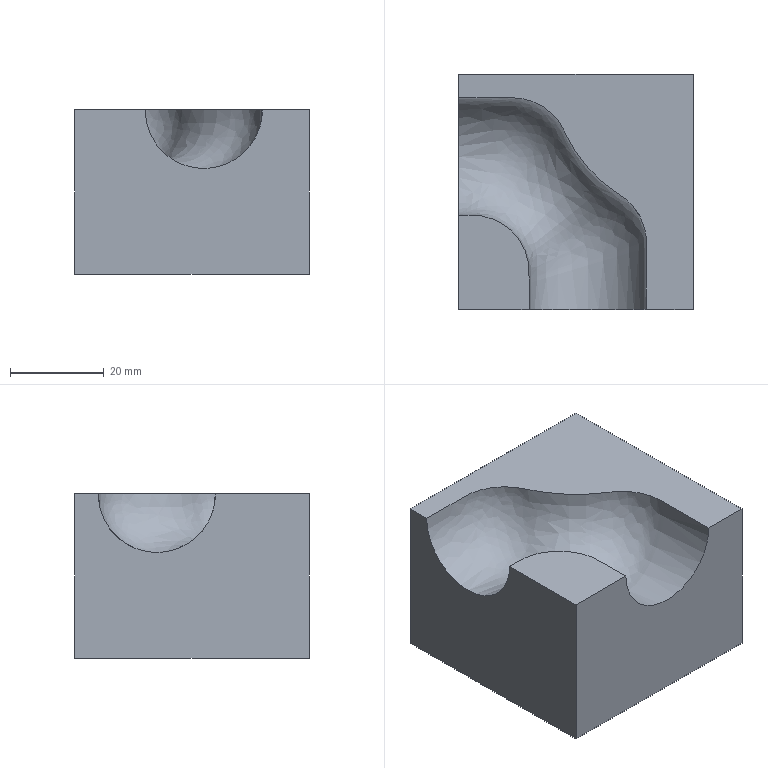Part | NX | 1 solid | 8 faces | box 50 x 50 x 35 mm | volume 75885 mm3 | plane 7 | spline 1
STEP:
#1=CARTESIAN_POINT('',(0.,45.,0.));
#2=VERTEX_POINT('',#1);
#3=CARTESIAN_POINT('',(0.,20.,0.));
#4=VERTEX_POINT('',#3);
#5=CARTESIAN_POINT('',(0.,45.,0.));
#6=CARTESIAN_POINT('',(0.,45.,-3.284));
#7=CARTESIAN_POINT('',(0.,42.295,-9.786));
#8=CARTESIAN_POINT('',(0.,32.5,-13.857));
#9=CARTESIAN_POINT('',(0.,22.705,-9.785));
#10=CARTESIAN_POINT('',(0.,20.,-3.285));
#11=CARTESIAN_POINT('',(0.,20.,0.));
#12=B_SPLINE_CURVE_WITH_KNOTS('',3,(#5,#6,#7,#8,#9,#10,#11),.UNSPECIFIED.,.F.,.F.,(4,1,1,1,4),(0.,0.25,0.5,0.75,1.),.UNSPECIFIED.);
#13=EDGE_CURVE('',#2,#4,#12,.T.);
#14=ORIENTED_EDGE('',*,*,#13,.F.);
#15=CARTESIAN_POINT('',(0.,50.,0.));
#16=VERTEX_POINT('',#15);
#17=CARTESIAN_POINT('',(0.,0.,0.));
#18=DIRECTION('',(0.,1.,0.));
#19=VECTOR('',#18,1000.);
#20=LINE('',#17,#19);
#21=EDGE_CURVE('',#2,#16,#20,.T.);
#22=ORIENTED_EDGE('',*,*,#21,.T.);
#23=CARTESIAN_POINT('',(0.,50.,-35.));
#24=VERTEX_POINT('',#23);
#25=CARTESIAN_POINT('',(0.,50.,-35.));
#26=DIRECTION('',(0.,0.,1.));
#27=VECTOR('',#26,1000.);
#28=LINE('',#25,#27);
#29=EDGE_CURVE('',#24,#16,#28,.T.);
#30=ORIENTED_EDGE('',*,*,#29,.F.);
#31=CARTESIAN_POINT('',(0.,0.,-35.));
#32=VERTEX_POINT('',#31);
#33=CARTESIAN_POINT('',(0.,0.,-35.));
#34=DIRECTION('',(0.,1.,0.));
#35=VECTOR('',#34,1000.);
#36=LINE('',#33,#35);
#37=EDGE_CURVE('',#32,#24,#36,.T.);
#38=ORIENTED_EDGE('',*,*,#37,.F.);
#39=CARTESIAN_POINT('',(0.,0.,0.));
#40=VERTEX_POINT('',#39);
#41=CARTESIAN_POINT('',(0.,0.,-35.));
#42=DIRECTION('',(0.,0.,1.));
#43=VECTOR('',#42,1000.);
#44=LINE('',#41,#43);
#45=EDGE_CURVE('',#32,#40,#44,.T.);
#46=ORIENTED_EDGE('',*,*,#45,.T.);
#47=CARTESIAN_POINT('',(0.,0.,0.));
#48=DIRECTION('',(0.,1.,0.));
#49=VECTOR('',#48,1000.);
#50=LINE('',#47,#49);
#51=EDGE_CURVE('',#40,#4,#50,.T.);
#52=ORIENTED_EDGE('',*,*,#51,.T.);
#53=EDGE_LOOP('',(#14,#22,#30,#38,#46,#52));
#54=FACE_BOUND('',#53,.T.);
#55=CARTESIAN_POINT('',(0.,0.,-35.));
#56=DIRECTION('',(1.,0.,0.));
#57=DIRECTION('',(0.,0.,-1.));
#58=AXIS2_PLACEMENT_3D('',#55,#56,#57);
#59=PLANE('',#58);
#60=ADVANCED_FACE('',(#54),#59,.F.);
#61=CARTESIAN_POINT('',(15.,0.,0.));
#62=VERTEX_POINT('',#61);
#63=CARTESIAN_POINT('',(40.,0.,0.));
#64=VERTEX_POINT('',#63);
#65=CARTESIAN_POINT('',(15.,0.,0.));
#66=CARTESIAN_POINT('',(15.,0.,-3.284));
#67=CARTESIAN_POINT('',(17.705,0.,-9.786));
#68=CARTESIAN_POINT('',(27.5,0.,-13.857));
#69=CARTESIAN_POINT('',(37.295,0.,-9.785));
#70=CARTESIAN_POINT('',(40.,0.,-3.285));
#71=CARTESIAN_POINT('',(40.,0.,0.));
#72=B_SPLINE_CURVE_WITH_KNOTS('',3,(#65,#66,#67,#68,#69,#70,#71),.UNSPECIFIED.,.F.,.F.,(4,1,1,1,4),(0.,0.25,0.5,0.75,1.),.UNSPECIFIED.);
#73=EDGE_CURVE('',#62,#64,#72,.T.);
#74=ORIENTED_EDGE('',*,*,#73,.F.);
#75=CARTESIAN_POINT('',(50.,0.,0.));
#76=DIRECTION('',(-1.,0.,0.));
#77=VECTOR('',#76,1000.);
#78=LINE('',#75,#77);
#79=EDGE_CURVE('',#62,#40,#78,.T.);
#80=ORIENTED_EDGE('',*,*,#79,.T.);
#81=ORIENTED_EDGE('',*,*,#45,.F.);
#82=CARTESIAN_POINT('',(50.,0.,-35.));
#83=VERTEX_POINT('',#82);
#84=CARTESIAN_POINT('',(50.,0.,-35.));
#85=DIRECTION('',(-1.,0.,0.));
#86=VECTOR('',#85,1000.);
#87=LINE('',#84,#86);
#88=EDGE_CURVE('',#83,#32,#87,.T.);
#89=ORIENTED_EDGE('',*,*,#88,.F.);
#90=CARTESIAN_POINT('',(50.,0.,0.));
#91=VERTEX_POINT('',#90);
#92=CARTESIAN_POINT('',(50.,0.,-35.));
#93=DIRECTION('',(0.,0.,1.));
#94=VECTOR('',#93,1000.);
#95=LINE('',#92,#94);
#96=EDGE_CURVE('',#83,#91,#95,.T.);
#97=ORIENTED_EDGE('',*,*,#96,.T.);
#98=CARTESIAN_POINT('',(50.,0.,0.));
#99=DIRECTION('',(-1.,0.,0.));
#100=VECTOR('',#99,1000.);
#101=LINE('',#98,#100);
#102=EDGE_CURVE('',#91,#64,#101,.T.);
#103=ORIENTED_EDGE('',*,*,#102,.T.);
#104=EDGE_LOOP('',(#74,#80,#81,#89,#97,#103));
#105=FACE_BOUND('',#104,.T.);
#106=CARTESIAN_POINT('',(50.,0.,-35.));
#107=DIRECTION('',(0.,1.,0.));
#108=DIRECTION('',(0.,0.,1.));
#109=AXIS2_PLACEMENT_3D('',#106,#107,#108);
#110=PLANE('',#109);
#111=ADVANCED_FACE('',(#105),#110,.F.);
#112=CARTESIAN_POINT('',(40.,0.,0.));
#113=CARTESIAN_POINT('',(40.,1.458,0.));
#114=CARTESIAN_POINT('',(39.999,4.376,0.));
#115=CARTESIAN_POINT('',(40.004,8.74,0.));
#116=CARTESIAN_POINT('',(39.987,12.414,0.));
#117=CARTESIAN_POINT('',(40.023,15.271,0.));
#118=CARTESIAN_POINT('',(39.51,18.133,0.));
#119=CARTESIAN_POINT('',(38.178,20.879,0.));
#120=CARTESIAN_POINT('',(36.19,23.093,0.));
#121=CARTESIAN_POINT('',(34.482,24.36,0.));
#122=CARTESIAN_POINT('',(32.637,25.485,0.));
#123=CARTESIAN_POINT('',(30.334,27.273,0.));
#124=CARTESIAN_POINT('',(27.665,29.806,0.));
#125=CARTESIAN_POINT('',(24.955,33.288,0.));
#126=CARTESIAN_POINT('',(23.146,36.496,0.));
#127=CARTESIAN_POINT('',(22.035,39.067,0.));
#128=CARTESIAN_POINT('',(20.341,41.437,0.));
#129=CARTESIAN_POINT('',(17.954,43.369,0.));
#130=CARTESIAN_POINT('',(15.201,44.519,0.));
#131=CARTESIAN_POINT('',(13.382,44.9,0.));
#132=CARTESIAN_POINT('',(12.299,44.987,0.));
#133=CARTESIAN_POINT('',(11.768,44.999,0.));
#134=CARTESIAN_POINT('',(11.654,45.,0.));
#135=CARTESIAN_POINT('',(11.403,45.,0.));
#136=CARTESIAN_POINT('',(11.323,45.,0.));
#137=CARTESIAN_POINT('',(10.876,45.,0.));
#138=CARTESIAN_POINT('',(10.783,45.,0.));
#139=CARTESIAN_POINT('',(10.487,45.,0.));
#140=CARTESIAN_POINT('',(10.089,45.,0.));
#141=CARTESIAN_POINT('',(9.59,45.,0.));
#142=CARTESIAN_POINT('',(9.175,45.,0.));
#143=CARTESIAN_POINT('',(8.953,45.,0.));
#144=CARTESIAN_POINT('',(8.694,45.,0.));
#145=CARTESIAN_POINT('',(8.757,45.,0.));
#146=CARTESIAN_POINT('',(8.722,45.,0.));
#147=CARTESIAN_POINT('',(8.699,45.,0.));
#148=CARTESIAN_POINT('',(8.596,45.,0.));
#149=CARTESIAN_POINT('',(8.419,45.,0.));
#150=CARTESIAN_POINT('',(8.089,45.,0.));
#151=CARTESIAN_POINT('',(7.511,45.,0.));
#152=CARTESIAN_POINT('',(6.231,45.,0.));
#153=CARTESIAN_POINT('',(3.964,45.,0.));
#154=CARTESIAN_POINT('',(1.44,45.,0.));
#155=CARTESIAN_POINT('',(0.,45.,0.));
#156=B_SPLINE_CURVE_WITH_KNOTS('',3,(#112,#113,#114,#115,#116,#117,#118,#119,#120,#121,#122,#123,#124,#125,#126,#127,#128,#129,#130,#131,#132,#133,#134,#135,#136,#137,#138,#139,#140,#141,#142,#143,#144,#145,#146,#147,#148,#149,#150,#151,#152,#153,#154,#155),.UNSPECIFIED.,.F.,.F.,(4,1,1,1,1,1,1,1,1,1,1,1,1,1,1,1,1,1,1,1,1,1,1,1,1,1,1,1,1,1,1,1,1,1,1,1,1,1,1,1,1,4),(0.,0.0625,0.125,0.1875,0.2188,0.25,0.3125,0.3438,0.375,0.4062,0.4375,0.5,0.5625,0.625,0.6562,0.6875,0.75,0.7812,0.8125,0.8281,0.832,0.834,0.8359,0.8398,0.8438,0.8477,0.8516,0.8594,0.8672,0.8711,0.873,0.875,0.877,0.8789,0.8828,0.8906,0.8984,0.9062,0.9219,0.9375,0.9688,1.),.UNSPECIFIED.);
#157=EDGE_CURVE('',#64,#2,#156,.T.);
#158=ORIENTED_EDGE('',*,*,#157,.F.);
#159=ORIENTED_EDGE('',*,*,#102,.F.);
#160=CARTESIAN_POINT('',(50.,50.,0.));
#161=VERTEX_POINT('',#160);
#162=CARTESIAN_POINT('',(50.,50.,0.));
#163=DIRECTION('',(0.,-1.,0.));
#164=VECTOR('',#163,1000.);
#165=LINE('',#162,#164);
#166=EDGE_CURVE('',#161,#91,#165,.T.);
#167=ORIENTED_EDGE('',*,*,#166,.F.);
#168=CARTESIAN_POINT('',(0.,50.,0.));
#169=DIRECTION('',(1.,0.,0.));
#170=VECTOR('',#169,1000.);
#171=LINE('',#168,#170);
#172=EDGE_CURVE('',#16,#161,#171,.T.);
#173=ORIENTED_EDGE('',*,*,#172,.F.);
#174=ORIENTED_EDGE('',*,*,#21,.F.);
#175=EDGE_LOOP('',(#158,#159,#167,#173,#174));
#176=FACE_BOUND('',#175,.T.);
#177=CARTESIAN_POINT('',(0.,0.,0.));
#178=DIRECTION('',(0.,0.,-1.));
#179=DIRECTION('',(-1.,0.,0.));
#180=AXIS2_PLACEMENT_3D('',#177,#178,#179);
#181=PLANE('',#180);
#182=ADVANCED_FACE('',(#176),#181,.F.);
#183=CARTESIAN_POINT('',(0.,20.,0.));
#184=CARTESIAN_POINT('',(0.6111,20.,0.));
#185=CARTESIAN_POINT('',(1.299,20.,0.));
#186=CARTESIAN_POINT('',(1.721,20.,0.));
#187=CARTESIAN_POINT('',(1.816,20.,0.));
#188=CARTESIAN_POINT('',(1.869,20.,0.));
#189=CARTESIAN_POINT('',(1.82,20.,0.));
#190=CARTESIAN_POINT('',(2.046,20.,0.));
#191=CARTESIAN_POINT('',(2.228,20.,0.));
#192=CARTESIAN_POINT('',(2.451,20.,0.));
#193=CARTESIAN_POINT('',(2.671,20.,0.));
#194=CARTESIAN_POINT('',(2.758,20.,0.));
#195=CARTESIAN_POINT('',(3.091,20.,0.));
#196=CARTESIAN_POINT('',(3.275,19.998,0.));
#197=CARTESIAN_POINT('',(4.143,19.968,0.));
#198=CARTESIAN_POINT('',(5.388,19.803,0.));
#199=CARTESIAN_POINT('',(7.194,19.298,0.));
#200=CARTESIAN_POINT('',(8.927,18.493,0.));
#201=CARTESIAN_POINT('',(11.094,17.03,0.));
#202=CARTESIAN_POINT('',(12.874,15.033,0.));
#203=CARTESIAN_POINT('',(14.073,12.756,0.));
#204=CARTESIAN_POINT('',(14.575,11.265,0.));
#205=CARTESIAN_POINT('',(14.825,10.105,0.));
#206=CARTESIAN_POINT('',(14.949,9.227,0.));
#207=CARTESIAN_POINT('',(14.992,8.526,0.));
#208=CARTESIAN_POINT('',(14.999,8.182,0.));
#209=CARTESIAN_POINT('',(15.,7.905,0.));
#210=CARTESIAN_POINT('',(15.,7.79,0.));
#211=CARTESIAN_POINT('',(15.,7.632,0.));
#212=CARTESIAN_POINT('',(15.,7.418,0.));
#213=CARTESIAN_POINT('',(15.,7.473,0.));
#214=CARTESIAN_POINT('',(15.,7.446,0.));
#215=CARTESIAN_POINT('',(15.,7.43,0.));
#216=CARTESIAN_POINT('',(15.,7.316,0.));
#217=CARTESIAN_POINT('',(15.,7.026,0.));
#218=CARTESIAN_POINT('',(15.,6.439,0.));
#219=CARTESIAN_POINT('',(15.,5.35,0.));
#220=CARTESIAN_POINT('',(15.,3.409,0.));
#221=CARTESIAN_POINT('',(15.,1.239,0.));
#222=CARTESIAN_POINT('',(15.,0.,0.));
#223=B_SPLINE_CURVE_WITH_KNOTS('',3,(#183,#184,#185,#186,#187,#188,#189,#190,#191,#192,#193,#194,#195,#196,#197,#198,#199,#200,#201,#202,#203,#204,#205,#206,#207,#208,#209,#210,#211,#212,#213,#214,#215,#216,#217,#218,#219,#220,#221,#222),.UNSPECIFIED.,.F.,.F.,(4,1,1,1,1,1,1,1,1,1,1,1,1,1,1,1,1,1,1,1,1,1,1,1,1,1,1,1,1,1,1,1,1,1,1,1,1,4),(0.,0.03125,0.04688,0.05469,0.05859,0.0625,0.06641,0.07031,0.07812,0.08594,0.09375,0.1016,0.1094,0.125,0.1875,0.25,0.3125,0.375,0.5,0.5625,0.625,0.6562,0.6875,0.7188,0.7266,0.7344,0.7422,0.7461,0.75,0.7539,0.7578,0.7656,0.7812,0.8125,0.8438,0.875,0.9375,1.),.UNSPECIFIED.);
#224=EDGE_CURVE('',#4,#62,#223,.T.);
#225=ORIENTED_EDGE('',*,*,#224,.F.);
#226=ORIENTED_EDGE('',*,*,#51,.F.);
#227=ORIENTED_EDGE('',*,*,#79,.F.);
#228=EDGE_LOOP('',(#225,#226,#227));
#229=FACE_BOUND('',#228,.T.);
#230=CARTESIAN_POINT('',(0.,0.,0.));
#231=DIRECTION('',(0.,0.,-1.));
#232=DIRECTION('',(-1.,0.,0.));
#233=AXIS2_PLACEMENT_3D('',#230,#231,#232);
#234=PLANE('',#233);
#235=ADVANCED_FACE('',(#229),#234,.F.);
#236=ORIENTED_EDGE('',*,*,#172,.T.);
#237=CARTESIAN_POINT('',(50.,50.,-35.));
#238=VERTEX_POINT('',#237);
#239=CARTESIAN_POINT('',(50.,50.,-35.));
#240=DIRECTION('',(0.,0.,1.));
#241=VECTOR('',#240,1000.);
#242=LINE('',#239,#241);
#243=EDGE_CURVE('',#238,#161,#242,.T.);
#244=ORIENTED_EDGE('',*,*,#243,.F.);
#245=CARTESIAN_POINT('',(0.,50.,-35.));
#246=DIRECTION('',(1.,0.,0.));
#247=VECTOR('',#246,1000.);
#248=LINE('',#245,#247);
#249=EDGE_CURVE('',#24,#238,#248,.T.);
#250=ORIENTED_EDGE('',*,*,#249,.F.);
#251=ORIENTED_EDGE('',*,*,#29,.T.);
#252=EDGE_LOOP('',(#236,#244,#250,#251));
#253=FACE_BOUND('',#252,.T.);
#254=CARTESIAN_POINT('',(0.,50.,-35.));
#255=DIRECTION('',(0.,-1.,0.));
#256=DIRECTION('',(0.,0.,-1.));
#257=AXIS2_PLACEMENT_3D('',#254,#255,#256);
#258=PLANE('',#257);
#259=ADVANCED_FACE('',(#253),#258,.F.);
#260=ORIENTED_EDGE('',*,*,#166,.T.);
#261=ORIENTED_EDGE('',*,*,#96,.F.);
#262=CARTESIAN_POINT('',(50.,50.,-35.));
#263=DIRECTION('',(0.,-1.,0.));
#264=VECTOR('',#263,1000.);
#265=LINE('',#262,#264);
#266=EDGE_CURVE('',#238,#83,#265,.T.);
#267=ORIENTED_EDGE('',*,*,#266,.F.);
#268=ORIENTED_EDGE('',*,*,#243,.T.);
#269=EDGE_LOOP('',(#260,#261,#267,#268));
#270=FACE_BOUND('',#269,.T.);
#271=CARTESIAN_POINT('',(50.,50.,-35.));
#272=DIRECTION('',(-1.,0.,0.));
#273=DIRECTION('',(0.,0.,1.));
#274=AXIS2_PLACEMENT_3D('',#271,#272,#273);
#275=PLANE('',#274);
#276=ADVANCED_FACE('',(#270),#275,.F.);
#277=ORIENTED_EDGE('',*,*,#37,.T.);
#278=ORIENTED_EDGE('',*,*,#249,.T.);
#279=ORIENTED_EDGE('',*,*,#266,.T.);
#280=ORIENTED_EDGE('',*,*,#88,.T.);
#281=EDGE_LOOP('',(#277,#278,#279,#280));
#282=FACE_BOUND('',#281,.T.);
#283=CARTESIAN_POINT('',(0.,0.,-35.));
#284=DIRECTION('',(0.,0.,-1.));
#285=DIRECTION('',(-1.,0.,0.));
#286=AXIS2_PLACEMENT_3D('',#283,#284,#285);
#287=PLANE('',#286);
#288=ADVANCED_FACE('',(#282),#287,.T.);
#289=ORIENTED_EDGE('',*,*,#73,.T.);
#290=ORIENTED_EDGE('',*,*,#157,.T.);
#291=ORIENTED_EDGE('',*,*,#13,.T.);
#292=ORIENTED_EDGE('',*,*,#224,.T.);
#293=EDGE_LOOP('',(#289,#290,#291,#292));
#294=FACE_BOUND('',#293,.T.);
#295=CARTESIAN_POINT('',(15.,0.,0.));
#296=CARTESIAN_POINT('',(15.,1.244,0.));
#297=CARTESIAN_POINT('',(15.,3.109,0.));
#298=CARTESIAN_POINT('',(15.,5.053,0.));
#299=CARTESIAN_POINT('',(15.,5.807,0.));
#300=CARTESIAN_POINT('',(15.,5.962,0.));
#301=CARTESIAN_POINT('',(15.,6.078,0.));
#302=CARTESIAN_POINT('',(15.,6.175,0.));
#303=CARTESIAN_POINT('',(15.,6.33,0.));
#304=CARTESIAN_POINT('',(15.,6.756,0.));
#305=CARTESIAN_POINT('',(15.,7.303,0.));
#306=CARTESIAN_POINT('',(15.,7.859,0.));
#307=CARTESIAN_POINT('',(15.,8.146,0.));
#308=CARTESIAN_POINT('',(14.991,8.57,0.));
#309=CARTESIAN_POINT('',(14.949,9.215,0.));
#310=CARTESIAN_POINT('',(14.848,9.946,0.));
#311=CARTESIAN_POINT('',(14.734,10.526,0.));
#312=CARTESIAN_POINT('',(14.665,10.821,0.));
#313=CARTESIAN_POINT('',(14.622,10.987,0.));
#314=CARTESIAN_POINT('',(14.61,11.033,0.));
#315=CARTESIAN_POINT('',(14.591,11.107,0.));
#316=CARTESIAN_POINT('',(14.556,11.237,0.));
#317=CARTESIAN_POINT('',(14.481,11.495,0.));
#318=CARTESIAN_POINT('',(14.317,12.012,0.));
#319=CARTESIAN_POINT('',(13.923,13.038,0.));
#320=CARTESIAN_POINT('',(13.173,14.464,0.));
#321=CARTESIAN_POINT('',(12.184,15.772,0.));
#322=CARTESIAN_POINT('',(11.269,16.715,0.));
#323=CARTESIAN_POINT('',(10.744,17.173,0.));
#324=CARTESIAN_POINT('',(10.424,17.428,0.));
#325=CARTESIAN_POINT('',(10.328,17.503,0.));
#326=CARTESIAN_POINT('',(10.23,17.577,0.));
#327=CARTESIAN_POINT('',(10.1,17.675,0.));
#328=CARTESIAN_POINT('',(9.935,17.794,0.));
#329=CARTESIAN_POINT('',(9.533,18.072,0.));
#330=CARTESIAN_POINT('',(8.914,18.457,0.));
#331=CARTESIAN_POINT('',(8.058,18.896,0.));
#332=CARTESIAN_POINT('',(7.183,19.26,0.));
#333=CARTESIAN_POINT('',(6.298,19.55,0.));
#334=CARTESIAN_POINT('',(5.559,19.731,0.));
#335=CARTESIAN_POINT('',(5.082,19.82,0.));
#336=CARTESIAN_POINT('',(4.862,19.855,0.));
#337=CARTESIAN_POINT('',(4.716,19.877,0.));
#338=CARTESIAN_POINT('',(4.315,19.933,0.));
#339=CARTESIAN_POINT('',(3.808,19.979,0.));
#340=CARTESIAN_POINT('',(3.306,19.998,0.));
#341=CARTESIAN_POINT('',(3.034,20.,0.));
#342=CARTESIAN_POINT('',(2.562,20.,0.));
#343=CARTESIAN_POINT('',(1.557,20.,0.));
#344=CARTESIAN_POINT('',(0.6219,20.,0.));
#345=CARTESIAN_POINT('',(0.,20.,0.));
#346=CARTESIAN_POINT('',(15.,0.,-3.125));
#347=CARTESIAN_POINT('',(15.,1.244,-3.125));
#348=CARTESIAN_POINT('',(15.,3.109,-3.157));
#349=CARTESIAN_POINT('',(15.,5.053,-3.237));
#350=CARTESIAN_POINT('',(15.,5.807,-3.274));
#351=CARTESIAN_POINT('',(15.,5.962,-3.282));
#352=CARTESIAN_POINT('',(15.,6.078,-3.288));
#353=CARTESIAN_POINT('',(15.,6.175,-3.293));
#354=CARTESIAN_POINT('',(15.,6.33,-3.299));
#355=CARTESIAN_POINT('',(15.,6.756,-3.314));
#356=CARTESIAN_POINT('',(15.,7.303,-3.319));
#357=CARTESIAN_POINT('',(15.,7.859,-3.305));
#358=CARTESIAN_POINT('',(15.,8.146,-3.294));
#359=CARTESIAN_POINT('',(14.991,8.57,-3.273));
#360=CARTESIAN_POINT('',(14.949,9.215,-3.224));
#361=CARTESIAN_POINT('',(14.848,9.946,-3.141));
#362=CARTESIAN_POINT('',(14.734,10.526,-3.06));
#363=CARTESIAN_POINT('',(14.665,10.821,-3.014));
#364=CARTESIAN_POINT('',(14.622,10.987,-2.988));
#365=CARTESIAN_POINT('',(14.61,11.033,-2.98));
#366=CARTESIAN_POINT('',(14.591,11.107,-2.968));
#367=CARTESIAN_POINT('',(14.556,11.237,-2.947));
#368=CARTESIAN_POINT('',(14.481,11.495,-2.906));
#369=CARTESIAN_POINT('',(14.317,12.012,-2.831));
#370=CARTESIAN_POINT('',(13.923,13.038,-2.711));
#371=CARTESIAN_POINT('',(13.173,14.464,-2.632));
#372=CARTESIAN_POINT('',(12.184,15.772,-2.683));
#373=CARTESIAN_POINT('',(11.269,16.715,-2.796));
#374=CARTESIAN_POINT('',(10.744,17.173,-2.879));
#375=CARTESIAN_POINT('',(10.424,17.428,-2.934));
#376=CARTESIAN_POINT('',(10.328,17.503,-2.951));
#377=CARTESIAN_POINT('',(10.23,17.577,-2.968));
#378=CARTESIAN_POINT('',(10.1,17.675,-2.991));
#379=CARTESIAN_POINT('',(9.935,17.794,-3.018));
#380=CARTESIAN_POINT('',(9.533,18.072,-3.081));
#381=CARTESIAN_POINT('',(8.914,18.457,-3.165));
#382=CARTESIAN_POINT('',(8.058,18.896,-3.249));
#383=CARTESIAN_POINT('',(7.183,19.26,-3.298));
#384=CARTESIAN_POINT('',(6.298,19.55,-3.312));
#385=CARTESIAN_POINT('',(5.559,19.731,-3.295));
#386=CARTESIAN_POINT('',(5.082,19.82,-3.272));
#387=CARTESIAN_POINT('',(4.862,19.855,-3.259));
#388=CARTESIAN_POINT('',(4.716,19.877,-3.249));
#389=CARTESIAN_POINT('',(4.315,19.933,-3.223));
#390=CARTESIAN_POINT('',(3.808,19.979,-3.196));
#391=CARTESIAN_POINT('',(3.306,19.998,-3.176));
#392=CARTESIAN_POINT('',(3.034,20.,-3.166));
#393=CARTESIAN_POINT('',(2.562,20.,-3.154));
#394=CARTESIAN_POINT('',(1.557,20.,-3.133));
#395=CARTESIAN_POINT('',(0.6219,20.,-3.125));
#396=CARTESIAN_POINT('',(0.,20.,-3.125));
#397=CARTESIAN_POINT('',(16.054,0.,-6.608));
#398=CARTESIAN_POINT('',(16.054,1.314,-6.608));
#399=CARTESIAN_POINT('',(16.054,3.286,-6.675));
#400=CARTESIAN_POINT('',(16.054,5.339,-6.844));
#401=CARTESIAN_POINT('',(16.054,6.137,-6.923));
#402=CARTESIAN_POINT('',(16.054,6.3,-6.94));
#403=CARTESIAN_POINT('',(16.054,6.423,-6.953));
#404=CARTESIAN_POINT('',(16.054,6.525,-6.963));
#405=CARTESIAN_POINT('',(16.054,6.688,-6.976));
#406=CARTESIAN_POINT('',(16.051,7.138,-7.008));
#407=CARTESIAN_POINT('',(16.042,7.714,-7.018));
#408=CARTESIAN_POINT('',(16.025,8.299,-6.989));
#409=CARTESIAN_POINT('',(16.013,8.602,-6.965));
#410=CARTESIAN_POINT('',(15.985,9.051,-6.921));
#411=CARTESIAN_POINT('',(15.908,9.73,-6.818));
#412=CARTESIAN_POINT('',(15.758,10.488,-6.642));
#413=CARTESIAN_POINT('',(15.603,11.082,-6.471));
#414=CARTESIAN_POINT('',(15.513,11.382,-6.374));
#415=CARTESIAN_POINT('',(15.458,11.551,-6.318));
#416=CARTESIAN_POINT('',(15.443,11.597,-6.302));
#417=CARTESIAN_POINT('',(15.418,11.672,-6.276));
#418=CARTESIAN_POINT('',(15.373,11.803,-6.231));
#419=CARTESIAN_POINT('',(15.279,12.065,-6.145));
#420=CARTESIAN_POINT('',(15.078,12.59,-5.987));
#421=CARTESIAN_POINT('',(14.615,13.638,-5.733));
#422=CARTESIAN_POINT('',(13.784,15.111,-5.566));
#423=CARTESIAN_POINT('',(12.742,16.487,-5.674));
#424=CARTESIAN_POINT('',(11.8,17.494,-5.912));
#425=CARTESIAN_POINT('',(11.268,17.991,-6.087));
#426=CARTESIAN_POINT('',(10.945,18.269,-6.204));
#427=CARTESIAN_POINT('',(10.848,18.352,-6.24));
#428=CARTESIAN_POINT('',(10.75,18.433,-6.277));
#429=CARTESIAN_POINT('',(10.619,18.54,-6.325));
#430=CARTESIAN_POINT('',(10.453,18.671,-6.382));
#431=CARTESIAN_POINT('',(10.047,18.976,-6.515));
#432=CARTESIAN_POINT('',(9.414,19.401,-6.694));
#433=CARTESIAN_POINT('',(8.526,19.887,-6.87));
#434=CARTESIAN_POINT('',(7.609,20.289,-6.974));
#435=CARTESIAN_POINT('',(6.673,20.603,-7.003));
#436=CARTESIAN_POINT('',(5.89,20.792,-6.967));
#437=CARTESIAN_POINT('',(5.385,20.881,-6.918));
#438=CARTESIAN_POINT('',(5.153,20.915,-6.891));
#439=CARTESIAN_POINT('',(4.998,20.937,-6.871));
#440=CARTESIAN_POINT('',(4.571,20.99,-6.816));
#441=CARTESIAN_POINT('',(4.032,21.034,-6.759));
#442=CARTESIAN_POINT('',(3.497,21.052,-6.716));
#443=CARTESIAN_POINT('',(3.206,21.055,-6.695));
#444=CARTESIAN_POINT('',(2.708,21.054,-6.67));
#445=CARTESIAN_POINT('',(1.645,21.055,-6.625));
#446=CARTESIAN_POINT('',(0.6571,21.054,-6.608));
#447=CARTESIAN_POINT('',(0.,21.054,-6.608));
#448=CARTESIAN_POINT('',(18.544,0.,-9.263));
#449=CARTESIAN_POINT('',(18.544,1.481,-9.263));
#450=CARTESIAN_POINT('',(18.544,3.702,-9.357));
#451=CARTESIAN_POINT('',(18.544,6.016,-9.593));
#452=CARTESIAN_POINT('',(18.544,6.915,-9.705));
#453=CARTESIAN_POINT('',(18.544,7.1,-9.728));
#454=CARTESIAN_POINT('',(18.544,7.238,-9.747));
#455=CARTESIAN_POINT('',(18.543,7.352,-9.76));
#456=CARTESIAN_POINT('',(18.542,7.534,-9.779));
#457=CARTESIAN_POINT('',(18.533,8.039,-9.823));
#458=CARTESIAN_POINT('',(18.501,8.686,-9.838));
#459=CARTESIAN_POINT('',(18.445,9.338,-9.797));
#460=CARTESIAN_POINT('',(18.405,9.681,-9.763));
#461=CARTESIAN_POINT('',(18.331,10.189,-9.701));
#462=CARTESIAN_POINT('',(18.171,10.947,-9.557));
#463=CARTESIAN_POINT('',(17.908,11.769,-9.31));
#464=CARTESIAN_POINT('',(17.657,12.397,-9.07));
#465=CARTESIAN_POINT('',(17.515,12.708,-8.935));
#466=CARTESIAN_POINT('',(17.431,12.881,-8.856));
#467=CARTESIAN_POINT('',(17.408,12.929,-8.834));
#468=CARTESIAN_POINT('',(17.37,13.006,-8.797));
#469=CARTESIAN_POINT('',(17.302,13.14,-8.734));
#470=CARTESIAN_POINT('',(17.163,13.41,-8.613));
#471=CARTESIAN_POINT('',(16.874,13.955,-8.392));
#472=CARTESIAN_POINT('',(16.249,15.055,-8.036));
#473=CARTESIAN_POINT('',(15.228,16.639,-7.801));
#474=CARTESIAN_POINT('',(14.058,18.174,-7.954));
#475=CARTESIAN_POINT('',(13.056,19.335,-8.288));
#476=CARTESIAN_POINT('',(12.505,19.922,-8.532));
#477=CARTESIAN_POINT('',(12.176,20.257,-8.697));
#478=CARTESIAN_POINT('',(12.077,20.356,-8.747));
#479=CARTESIAN_POINT('',(11.978,20.454,-8.799));
#480=CARTESIAN_POINT('',(11.846,20.583,-8.866));
#481=CARTESIAN_POINT('',(11.676,20.741,-8.946));
#482=CARTESIAN_POINT('',(11.259,21.111,-9.133));
#483=CARTESIAN_POINT('',(10.594,21.63,-9.383));
#484=CARTESIAN_POINT('',(9.632,22.228,-9.63));
#485=CARTESIAN_POINT('',(8.612,22.718,-9.776));
#486=CARTESIAN_POINT('',(7.559,23.089,-9.817));
#487=CARTESIAN_POINT('',(6.672,23.298,-9.766));
#488=CARTESIAN_POINT('',(6.1,23.387,-9.697));
#489=CARTESIAN_POINT('',(5.838,23.419,-9.659));
#490=CARTESIAN_POINT('',(5.663,23.438,-9.631));
#491=CARTESIAN_POINT('',(5.175,23.486,-9.554));
#492=CARTESIAN_POINT('',(4.56,23.525,-9.474));
#493=CARTESIAN_POINT('',(3.949,23.542,-9.414));
#494=CARTESIAN_POINT('',(3.612,23.544,-9.385));
#495=CARTESIAN_POINT('',(3.052,23.543,-9.349));
#496=CARTESIAN_POINT('',(1.853,23.544,-9.286));
#497=CARTESIAN_POINT('',(0.7404,23.544,-9.263));
#498=CARTESIAN_POINT('',(0.,23.544,-9.263));
#499=CARTESIAN_POINT('',(23.956,0.,-12.388));
#500=CARTESIAN_POINT('',(23.956,1.843,-12.388));
#501=CARTESIAN_POINT('',(23.956,4.607,-12.514));
#502=CARTESIAN_POINT('',(23.956,7.486,-12.83));
#503=CARTESIAN_POINT('',(23.956,8.607,-12.979));
#504=CARTESIAN_POINT('',(23.956,8.837,-13.01));
#505=CARTESIAN_POINT('',(23.956,9.01,-13.035));
#506=CARTESIAN_POINT('',(23.956,9.151,-13.053));
#507=CARTESIAN_POINT('',(23.952,9.374,-13.077));
#508=CARTESIAN_POINT('',(23.929,9.999,-13.137));
#509=CARTESIAN_POINT('',(23.849,10.798,-13.157));
#510=CARTESIAN_POINT('',(23.706,11.596,-13.102));
#511=CARTESIAN_POINT('',(23.606,12.026,-13.057));
#512=CARTESIAN_POINT('',(23.433,12.662,-12.974));
#513=CARTESIAN_POINT('',(23.092,13.592,-12.781));
#514=CARTESIAN_POINT('',(22.583,14.554,-12.45));
#515=CARTESIAN_POINT('',(22.121,15.255,-12.13));
#516=CARTESIAN_POINT('',(21.868,15.591,-11.95));
#517=CARTESIAN_POINT('',(21.722,15.774,-11.843));
#518=CARTESIAN_POINT('',(21.681,15.824,-11.814));
#519=CARTESIAN_POINT('',(21.615,15.905,-11.765));
#520=CARTESIAN_POINT('',(21.496,16.048,-11.681));
#521=CARTESIAN_POINT('',(21.259,16.336,-11.519));
#522=CARTESIAN_POINT('',(20.779,16.923,-11.223));
#523=CARTESIAN_POINT('',(19.801,18.135,-10.747));
#524=CARTESIAN_POINT('',(18.366,19.96,-10.433));
#525=CARTESIAN_POINT('',(16.92,21.842,-10.637));
#526=CARTESIAN_POINT('',(15.785,23.338,-11.084));
#527=CARTESIAN_POINT('',(15.194,24.121,-11.411));
#528=CARTESIAN_POINT('',(14.851,24.577,-11.631));
#529=CARTESIAN_POINT('',(14.749,24.713,-11.698));
#530=CARTESIAN_POINT('',(14.648,24.848,-11.767));
#531=CARTESIAN_POINT('',(14.512,25.025,-11.857));
#532=CARTESIAN_POINT('',(14.337,25.241,-11.964));
#533=CARTESIAN_POINT('',(13.896,25.751,-12.214));
#534=CARTESIAN_POINT('',(13.159,26.477,-12.548));
#535=CARTESIAN_POINT('',(12.034,27.319,-12.878));
#536=CARTESIAN_POINT('',(10.795,28.,-13.074));
#537=CARTESIAN_POINT('',(9.484,28.495,-13.129));
#538=CARTESIAN_POINT('',(8.371,28.748,-13.061));
#539=CARTESIAN_POINT('',(7.655,28.836,-12.969));
#540=CARTESIAN_POINT('',(7.329,28.863,-12.918));
#541=CARTESIAN_POINT('',(7.109,28.878,-12.881));
#542=CARTESIAN_POINT('',(6.489,28.913,-12.778));
#543=CARTESIAN_POINT('',(5.708,28.943,-12.671));
#544=CARTESIAN_POINT('',(4.93,28.955,-12.59));
#545=CARTESIAN_POINT('',(4.495,28.957,-12.551));
#546=CARTESIAN_POINT('',(3.8,28.956,-12.504));
#547=CARTESIAN_POINT('',(2.306,28.957,-12.419));
#548=CARTESIAN_POINT('',(0.9214,28.956,-12.388));
#549=CARTESIAN_POINT('',(0.,28.956,-12.388));
#550=CARTESIAN_POINT('',(27.5,0.,-13.216));
#551=CARTESIAN_POINT('',(27.5,2.08,-13.216));
#552=CARTESIAN_POINT('',(27.5,5.2,-13.351));
#553=CARTESIAN_POINT('',(27.5,8.449,-13.688));
#554=CARTESIAN_POINT('',(27.5,9.715,-13.847));
#555=CARTESIAN_POINT('',(27.5,9.975,-13.881));
#556=CARTESIAN_POINT('',(27.5,10.17,-13.907));
#557=CARTESIAN_POINT('',(27.499,10.329,-13.926));
#558=CARTESIAN_POINT('',(27.493,10.578,-13.952));
#559=CARTESIAN_POINT('',(27.462,11.281,-14.016));
#560=CARTESIAN_POINT('',(27.35,12.181,-14.037));
#561=CARTESIAN_POINT('',(27.15,13.074,-13.979));
#562=CARTESIAN_POINT('',(27.011,13.561,-13.93));
#563=CARTESIAN_POINT('',(26.774,14.281,-13.841));
#564=CARTESIAN_POINT('',(26.314,15.324,-13.636));
#565=CARTESIAN_POINT('',(25.643,16.377,-13.283));
#566=CARTESIAN_POINT('',(25.043,17.126,-12.941));
#567=CARTESIAN_POINT('',(24.719,17.478,-12.749));
#568=CARTESIAN_POINT('',(24.531,17.668,-12.636));
#569=CARTESIAN_POINT('',(24.479,17.72,-12.604));
#570=CARTESIAN_POINT('',(24.394,17.803,-12.552));
#571=CARTESIAN_POINT('',(24.243,17.951,-12.462));
#572=CARTESIAN_POINT('',(23.941,18.251,-12.29));
#573=CARTESIAN_POINT('',(23.336,18.866,-11.974));
#574=CARTESIAN_POINT('',(22.127,20.152,-11.466));
#575=CARTESIAN_POINT('',(20.42,22.135,-11.131));
#576=CARTESIAN_POINT('',(18.794,24.243,-11.349));
#577=CARTESIAN_POINT('',(17.571,25.958,-11.825));
#578=CARTESIAN_POINT('',(16.954,26.87,-12.174));
#579=CARTESIAN_POINT('',(16.603,27.406,-12.409));
#580=CARTESIAN_POINT('',(16.498,27.566,-12.481));
#581=CARTESIAN_POINT('',(16.396,27.725,-12.554));
#582=CARTESIAN_POINT('',(16.258,27.932,-12.65));
#583=CARTESIAN_POINT('',(16.079,28.187,-12.765));
#584=CARTESIAN_POINT('',(15.622,28.79,-13.031));
#585=CARTESIAN_POINT('',(14.839,29.651,-13.387));
#586=CARTESIAN_POINT('',(13.607,30.652,-13.74));
#587=CARTESIAN_POINT('',(12.225,31.458,-13.949));
#588=CARTESIAN_POINT('',(10.745,32.035,-14.007));
#589=CARTESIAN_POINT('',(9.484,32.315,-13.935));
#590=CARTESIAN_POINT('',(8.674,32.404,-13.836));
#591=CARTESIAN_POINT('',(8.304,32.428,-13.782));
#592=CARTESIAN_POINT('',(8.055,32.439,-13.742));
#593=CARTESIAN_POINT('',(7.349,32.466,-13.632));
#594=CARTESIAN_POINT('',(6.46,32.489,-13.518));
#595=CARTESIAN_POINT('',(5.572,32.499,-13.432));
#596=CARTESIAN_POINT('',(5.072,32.5,-13.39));
#597=CARTESIAN_POINT('',(4.29,32.5,-13.34));
#598=CARTESIAN_POINT('',(2.602,32.5,-13.249));
#599=CARTESIAN_POINT('',(1.04,32.5,-13.216));
#600=CARTESIAN_POINT('',(0.,32.5,-13.216));
#601=CARTESIAN_POINT('',(31.044,0.,-12.388));
#602=CARTESIAN_POINT('',(31.044,2.317,-12.388));
#603=CARTESIAN_POINT('',(31.044,5.792,-12.514));
#604=CARTESIAN_POINT('',(31.044,9.412,-12.83));
#605=CARTESIAN_POINT('',(31.044,10.823,-12.979));
#606=CARTESIAN_POINT('',(31.044,11.112,-13.01));
#607=CARTESIAN_POINT('',(31.044,11.33,-13.035));
#608=CARTESIAN_POINT('',(31.042,11.506,-13.053));
#609=CARTESIAN_POINT('',(31.035,11.783,-13.077));
#610=CARTESIAN_POINT('',(30.995,12.564,-13.137));
#611=CARTESIAN_POINT('',(30.852,13.564,-13.157));
#612=CARTESIAN_POINT('',(30.595,14.552,-13.102));
#613=CARTESIAN_POINT('',(30.416,15.097,-13.057));
#614=CARTESIAN_POINT('',(30.114,15.9,-12.974));
#615=CARTESIAN_POINT('',(29.536,17.056,-12.781));
#616=CARTESIAN_POINT('',(28.704,18.2,-12.45));
#617=CARTESIAN_POINT('',(27.966,18.997,-12.13));
#618=CARTESIAN_POINT('',(27.569,19.365,-11.95));
#619=CARTESIAN_POINT('',(27.341,19.562,-11.843));
#620=CARTESIAN_POINT('',(27.277,19.615,-11.814));
#621=CARTESIAN_POINT('',(27.174,19.701,-11.765));
#622=CARTESIAN_POINT('',(26.989,19.855,-11.681));
#623=CARTESIAN_POINT('',(26.623,20.166,-11.519));
#624=CARTESIAN_POINT('',(25.892,20.809,-11.223));
#625=CARTESIAN_POINT('',(24.453,22.169,-10.747));
#626=CARTESIAN_POINT('',(22.475,24.31,-10.433));
#627=CARTESIAN_POINT('',(20.668,26.645,-10.637));
#628=CARTESIAN_POINT('',(19.358,28.579,-11.084));
#629=CARTESIAN_POINT('',(18.715,29.62,-11.411));
#630=CARTESIAN_POINT('',(18.354,30.235,-11.631));
#631=CARTESIAN_POINT('',(18.247,30.419,-11.698));
#632=CARTESIAN_POINT('',(18.143,30.602,-11.767));
#633=CARTESIAN_POINT('',(18.004,30.84,-11.857));
#634=CARTESIAN_POINT('',(17.82,31.133,-11.964));
#635=CARTESIAN_POINT('',(17.347,31.828,-12.214));
#636=CARTESIAN_POINT('',(16.519,32.824,-12.548));
#637=CARTESIAN_POINT('',(15.18,33.985,-12.878));
#638=CARTESIAN_POINT('',(13.654,34.916,-13.074));
#639=CARTESIAN_POINT('',(12.006,35.574,-13.129));
#640=CARTESIAN_POINT('',(10.597,35.883,-13.061));
#641=CARTESIAN_POINT('',(9.692,35.971,-12.969));
#642=CARTESIAN_POINT('',(9.28,35.992,-12.918));
#643=CARTESIAN_POINT('',(9.002,36.,-12.881));
#644=CARTESIAN_POINT('',(8.209,36.02,-12.778));
#645=CARTESIAN_POINT('',(7.212,36.036,-12.671));
#646=CARTESIAN_POINT('',(6.215,36.043,-12.59));
#647=CARTESIAN_POINT('',(5.65,36.044,-12.551));
#648=CARTESIAN_POINT('',(4.78,36.043,-12.504));
#649=CARTESIAN_POINT('',(2.899,36.044,-12.419));
#650=CARTESIAN_POINT('',(1.158,36.044,-12.388));
#651=CARTESIAN_POINT('',(0.,36.044,-12.388));
#652=CARTESIAN_POINT('',(36.456,0.,-9.263));
#653=CARTESIAN_POINT('',(36.456,2.679,-9.263));
#654=CARTESIAN_POINT('',(36.456,6.697,-9.357));
#655=CARTESIAN_POINT('',(36.456,10.883,-9.593));
#656=CARTESIAN_POINT('',(36.456,12.515,-9.705));
#657=CARTESIAN_POINT('',(36.456,12.85,-9.728));
#658=CARTESIAN_POINT('',(36.457,13.102,-9.747));
#659=CARTESIAN_POINT('',(36.455,13.305,-9.76));
#660=CARTESIAN_POINT('',(36.445,13.622,-9.779));
#661=CARTESIAN_POINT('',(36.391,14.523,-9.823));
#662=CARTESIAN_POINT('',(36.2,15.676,-9.838));
#663=CARTESIAN_POINT('',(35.856,16.81,-9.797));
#664=CARTESIAN_POINT('',(35.617,17.442,-9.763));
#665=CARTESIAN_POINT('',(35.216,18.373,-9.701));
#666=CARTESIAN_POINT('',(34.457,19.701,-9.557));
#667=CARTESIAN_POINT('',(33.379,20.985,-9.31));
#668=CARTESIAN_POINT('',(32.43,21.855,-9.07));
#669=CARTESIAN_POINT('',(31.922,22.248,-8.935));
#670=CARTESIAN_POINT('',(31.631,22.454,-8.856));
#671=CARTESIAN_POINT('',(31.55,22.511,-8.834));
#672=CARTESIAN_POINT('',(31.419,22.601,-8.797));
#673=CARTESIAN_POINT('',(31.183,22.763,-8.734));
#674=CARTESIAN_POINT('',(30.719,23.091,-8.613));
#675=CARTESIAN_POINT('',(29.798,23.776,-8.392));
#676=CARTESIAN_POINT('',(28.005,25.249,-8.036));
#677=CARTESIAN_POINT('',(25.613,27.632,-7.801));
#678=CARTESIAN_POINT('',(23.53,30.313,-7.954));
#679=CARTESIAN_POINT('',(22.087,32.581,-8.288));
#680=CARTESIAN_POINT('',(21.404,33.818,-8.532));
#681=CARTESIAN_POINT('',(21.03,34.555,-8.697));
#682=CARTESIAN_POINT('',(20.919,34.777,-8.747));
#683=CARTESIAN_POINT('',(20.813,34.996,-8.799));
#684=CARTESIAN_POINT('',(20.671,35.282,-8.866));
#685=CARTESIAN_POINT('',(20.481,35.633,-8.946));
#686=CARTESIAN_POINT('',(19.984,36.469,-9.133));
#687=CARTESIAN_POINT('',(19.085,37.671,-9.383));
#688=CARTESIAN_POINT('',(17.583,39.075,-9.63));
#689=CARTESIAN_POINT('',(15.837,40.197,-9.776));
#690=CARTESIAN_POINT('',(13.932,40.98,-9.817));
#691=CARTESIAN_POINT('',(12.297,41.332,-9.766));
#692=CARTESIAN_POINT('',(11.248,41.42,-9.697));
#693=CARTESIAN_POINT('',(10.771,41.436,-9.659));
#694=CARTESIAN_POINT('',(10.448,41.439,-9.631));
#695=CARTESIAN_POINT('',(9.523,41.447,-9.554));
#696=CARTESIAN_POINT('',(8.36,41.453,-9.474));
#697=CARTESIAN_POINT('',(7.196,41.456,-9.414));
#698=CARTESIAN_POINT('',(6.532,41.456,-9.385));
#699=CARTESIAN_POINT('',(5.528,41.456,-9.349));
#700=CARTESIAN_POINT('',(3.351,41.456,-9.286));
#701=CARTESIAN_POINT('',(1.339,41.456,-9.263));
#702=CARTESIAN_POINT('',(0.,41.456,-9.263));
#703=CARTESIAN_POINT('',(38.946,0.,-6.608));
#704=CARTESIAN_POINT('',(38.946,2.845,-6.608));
#705=CARTESIAN_POINT('',(38.946,7.114,-6.675));
#706=CARTESIAN_POINT('',(38.946,11.56,-6.844));
#707=CARTESIAN_POINT('',(38.946,13.293,-6.923));
#708=CARTESIAN_POINT('',(38.946,13.649,-6.94));
#709=CARTESIAN_POINT('',(38.946,13.916,-6.953));
#710=CARTESIAN_POINT('',(38.944,14.132,-6.963));
#711=CARTESIAN_POINT('',(38.933,14.468,-6.976));
#712=CARTESIAN_POINT('',(38.872,15.425,-7.008));
#713=CARTESIAN_POINT('',(38.659,16.647,-7.018));
#714=CARTESIAN_POINT('',(38.276,17.849,-6.989));
#715=CARTESIAN_POINT('',(38.009,18.52,-6.965));
#716=CARTESIAN_POINT('',(37.563,19.511,-6.921));
#717=CARTESIAN_POINT('',(36.72,20.918,-6.818));
#718=CARTESIAN_POINT('',(35.529,22.266,-6.642));
#719=CARTESIAN_POINT('',(34.483,23.169,-6.471));
#720=CARTESIAN_POINT('',(33.924,23.574,-6.374));
#721=CARTESIAN_POINT('',(33.605,23.785,-6.318));
#722=CARTESIAN_POINT('',(33.516,23.842,-6.302));
#723=CARTESIAN_POINT('',(33.371,23.934,-6.276));
#724=CARTESIAN_POINT('',(33.112,24.1,-6.231));
#725=CARTESIAN_POINT('',(32.603,24.437,-6.145));
#726=CARTESIAN_POINT('',(31.594,25.141,-5.987));
#727=CARTESIAN_POINT('',(29.639,26.666,-5.733));
#728=CARTESIAN_POINT('',(27.056,29.159,-5.566));
#729=CARTESIAN_POINT('',(24.847,32.,-5.674));
#730=CARTESIAN_POINT('',(23.342,34.422,-5.912));
#731=CARTESIAN_POINT('',(22.641,35.75,-6.087));
#732=CARTESIAN_POINT('',(22.26,36.543,-6.204));
#733=CARTESIAN_POINT('',(22.148,36.781,-6.24));
#734=CARTESIAN_POINT('',(22.041,37.017,-6.277));
#735=CARTESIAN_POINT('',(21.897,37.325,-6.325));
#736=CARTESIAN_POINT('',(21.704,37.703,-6.382));
#737=CARTESIAN_POINT('',(21.196,38.603,-6.515));
#738=CARTESIAN_POINT('',(20.265,39.9,-6.694));
#739=CARTESIAN_POINT('',(18.688,41.417,-6.87));
#740=CARTESIAN_POINT('',(16.841,42.626,-6.974));
#741=CARTESIAN_POINT('',(14.818,43.466,-7.003));
#742=CARTESIAN_POINT('',(13.078,43.838,-6.967));
#743=CARTESIAN_POINT('',(11.963,43.926,-6.918));
#744=CARTESIAN_POINT('',(11.456,43.94,-6.891));
#745=CARTESIAN_POINT('',(11.113,43.94,-6.871));
#746=CARTESIAN_POINT('',(10.127,43.943,-6.816));
#747=CARTESIAN_POINT('',(8.888,43.945,-6.759));
#748=CARTESIAN_POINT('',(7.647,43.946,-6.716));
#749=CARTESIAN_POINT('',(6.938,43.946,-6.695));
#750=CARTESIAN_POINT('',(5.872,43.946,-6.67));
#751=CARTESIAN_POINT('',(3.559,43.946,-6.625));
#752=CARTESIAN_POINT('',(1.423,43.946,-6.608));
#753=CARTESIAN_POINT('',(0.,43.946,-6.608));
#754=CARTESIAN_POINT('',(40.,0.,-3.125));
#755=CARTESIAN_POINT('',(40.,2.916,-3.125));
#756=CARTESIAN_POINT('',(40.,7.29,-3.157));
#757=CARTESIAN_POINT('',(40.,11.846,-3.237));
#758=CARTESIAN_POINT('',(40.,13.623,-3.274));
#759=CARTESIAN_POINT('',(40.,13.987,-3.282));
#760=CARTESIAN_POINT('',(40.,14.262,-3.288));
#761=CARTESIAN_POINT('',(39.998,14.482,-3.293));
#762=CARTESIAN_POINT('',(39.987,14.827,-3.299));
#763=CARTESIAN_POINT('',(39.923,15.806,-3.314));
#764=CARTESIAN_POINT('',(39.701,17.059,-3.319));
#765=CARTESIAN_POINT('',(39.301,18.289,-3.305));
#766=CARTESIAN_POINT('',(39.022,18.977,-3.294));
#767=CARTESIAN_POINT('',(38.557,19.992,-3.273));
#768=CARTESIAN_POINT('',(37.679,21.433,-3.224));
#769=CARTESIAN_POINT('',(36.439,22.808,-3.141));
#770=CARTESIAN_POINT('',(35.352,23.726,-3.06));
#771=CARTESIAN_POINT('',(34.772,24.135,-3.014));
#772=CARTESIAN_POINT('',(34.441,24.348,-2.988));
#773=CARTESIAN_POINT('',(34.348,24.406,-2.98));
#774=CARTESIAN_POINT('',(34.198,24.499,-2.968));
#775=CARTESIAN_POINT('',(33.929,24.666,-2.947));
#776=CARTESIAN_POINT('',(33.401,25.006,-2.906));
#777=CARTESIAN_POINT('',(32.354,25.719,-2.831));
#778=CARTESIAN_POINT('',(30.33,27.266,-2.711));
#779=CARTESIAN_POINT('',(27.668,29.806,-2.632));
#780=CARTESIAN_POINT('',(25.404,32.714,-2.683));
#781=CARTESIAN_POINT('',(23.874,35.202,-2.796));
#782=CARTESIAN_POINT('',(23.164,36.568,-2.879));
#783=CARTESIAN_POINT('',(22.781,37.384,-2.934));
#784=CARTESIAN_POINT('',(22.669,37.629,-2.951));
#785=CARTESIAN_POINT('',(22.561,37.873,-2.968));
#786=CARTESIAN_POINT('',(22.417,38.19,-2.991));
#787=CARTESIAN_POINT('',(22.222,38.58,-3.018));
#788=CARTESIAN_POINT('',(21.71,39.507,-3.081));
#789=CARTESIAN_POINT('',(20.765,40.845,-3.165));
#790=CARTESIAN_POINT('',(19.156,42.408,-3.249));
#791=CARTESIAN_POINT('',(17.266,43.655,-3.298));
#792=CARTESIAN_POINT('',(15.193,44.519,-3.312));
#793=CARTESIAN_POINT('',(13.409,44.899,-3.295));
#794=CARTESIAN_POINT('',(12.266,44.988,-3.272));
#795=CARTESIAN_POINT('',(11.747,45.,-3.259));
#796=CARTESIAN_POINT('',(11.395,45.,-3.249));
#797=CARTESIAN_POINT('',(10.383,45.,-3.223));
#798=CARTESIAN_POINT('',(9.112,45.,-3.196));
#799=CARTESIAN_POINT('',(7.838,45.,-3.176));
#800=CARTESIAN_POINT('',(7.11,45.,-3.166));
#801=CARTESIAN_POINT('',(6.017,45.,-3.154));
#802=CARTESIAN_POINT('',(3.648,45.,-3.133));
#803=CARTESIAN_POINT('',(1.458,45.,-3.125));
#804=CARTESIAN_POINT('',(0.,45.,-3.125));
#805=CARTESIAN_POINT('',(40.,0.,0.));
#806=CARTESIAN_POINT('',(40.,2.916,0.));
#807=CARTESIAN_POINT('',(40.,7.29,0.));
#808=CARTESIAN_POINT('',(40.,11.846,0.));
#809=CARTESIAN_POINT('',(40.,13.623,0.));
#810=CARTESIAN_POINT('',(40.,13.987,0.));
#811=CARTESIAN_POINT('',(40.,14.262,0.));
#812=CARTESIAN_POINT('',(39.998,14.482,0.));
#813=CARTESIAN_POINT('',(39.987,14.827,0.));
#814=CARTESIAN_POINT('',(39.923,15.806,0.));
#815=CARTESIAN_POINT('',(39.701,17.059,0.));
#816=CARTESIAN_POINT('',(39.301,18.289,0.));
#817=CARTESIAN_POINT('',(39.022,18.977,0.));
#818=CARTESIAN_POINT('',(38.557,19.992,0.));
#819=CARTESIAN_POINT('',(37.679,21.433,0.));
#820=CARTESIAN_POINT('',(36.439,22.808,0.));
#821=CARTESIAN_POINT('',(35.352,23.726,0.));
#822=CARTESIAN_POINT('',(34.772,24.135,0.));
#823=CARTESIAN_POINT('',(34.441,24.348,0.));
#824=CARTESIAN_POINT('',(34.348,24.406,0.));
#825=CARTESIAN_POINT('',(34.198,24.499,0.));
#826=CARTESIAN_POINT('',(33.929,24.666,0.));
#827=CARTESIAN_POINT('',(33.401,25.006,0.));
#828=CARTESIAN_POINT('',(32.354,25.719,0.));
#829=CARTESIAN_POINT('',(30.33,27.266,0.));
#830=CARTESIAN_POINT('',(27.668,29.806,0.));
#831=CARTESIAN_POINT('',(25.404,32.714,0.));
#832=CARTESIAN_POINT('',(23.874,35.202,0.));
#833=CARTESIAN_POINT('',(23.164,36.568,0.));
#834=CARTESIAN_POINT('',(22.781,37.384,0.));
#835=CARTESIAN_POINT('',(22.669,37.629,0.));
#836=CARTESIAN_POINT('',(22.561,37.873,0.));
#837=CARTESIAN_POINT('',(22.417,38.19,0.));
#838=CARTESIAN_POINT('',(22.222,38.58,0.));
#839=CARTESIAN_POINT('',(21.71,39.507,0.));
#840=CARTESIAN_POINT('',(20.765,40.845,0.));
#841=CARTESIAN_POINT('',(19.156,42.408,0.));
#842=CARTESIAN_POINT('',(17.266,43.655,0.));
#843=CARTESIAN_POINT('',(15.193,44.519,0.));
#844=CARTESIAN_POINT('',(13.409,44.899,0.));
#845=CARTESIAN_POINT('',(12.266,44.988,0.));
#846=CARTESIAN_POINT('',(11.747,45.,0.));
#847=CARTESIAN_POINT('',(11.395,45.,0.));
#848=CARTESIAN_POINT('',(10.383,45.,0.));
#849=CARTESIAN_POINT('',(9.112,45.,0.));
#850=CARTESIAN_POINT('',(7.838,45.,0.));
#851=CARTESIAN_POINT('',(7.11,45.,0.));
#852=CARTESIAN_POINT('',(6.017,45.,0.));
#853=CARTESIAN_POINT('',(3.648,45.,0.));
#854=CARTESIAN_POINT('',(1.458,45.,0.));
#855=CARTESIAN_POINT('',(0.,45.,0.));
#856=(BOUNDED_SURFACE()B_SPLINE_SURFACE(4,3,((#295,#296,#297,#298,#299,#300,#301,#302,#303,#304,#305,#306,#307,#308,#309,#310,#311,#312,#313,#314,#315,#316,#317,#318,#319,#320,#321,#322,#323,#324,#325,#326,#327,#328,#329,#330,#331,#332,#333,#334,#335,#336,#337,#338,#339,#340,#341,#342,#343,#344,#345),(#346,#347,#348,#349,#350,#351,#352,#353,#354,#355,#356,#357,#358,#359,#360,#361,#362,#363,#364,#365,#366,#367,#368,#369,#370,#371,#372,#373,#374,#375,#376,#377,#378,#379,#380,#381,#382,#383,#384,#385,#386,#387,#388,#389,#390,#391,#392,#393,#394,#395,#396),(#397,#398,#399,#400,#401,#402,#403,#404,#405,#406,#407,#408,#409,#410,#411,#412,#413,#414,#415,#416,#417,#418,#419,#420,#421,#422,#423,#424,#425,#426,#427,#428,#429,#430,#431,#432,#433,#434,#435,#436,#437,#438,#439,#440,#441,#442,#443,#444,#445,#446,#447),(#448,#449,#450,#451,#452,#453,#454,#455,#456,#457,#458,#459,#460,#461,#462,#463,#464,#465,#466,#467,#468,#469,#470,#471,#472,#473,#474,#475,#476,#477,#478,#479,#480,#481,#482,#483,#484,#485,#486,#487,#488,#489,#490,#491,#492,#493,#494,#495,#496,#497,#498),(#499,#500,#501,#502,#503,#504,#505,#506,#507,#508,#509,#510,#511,#512,#513,#514,#515,#516,#517,#518,#519,#520,#521,#522,#523,#524,#525,#526,#527,#528,#529,#530,#531,#532,#533,#534,#535,#536,#537,#538,#539,#540,#541,#542,#543,#544,#545,#546,#547,#548,#549),(#550,#551,#552,#553,#554,#555,#556,#557,#558,#559,#560,#561,#562,#563,#564,#565,#566,#567,#568,#569,#570,#571,#572,#573,#574,#575,#576,#577,#578,#579,#580,#581,#582,#583,#584,#585,#586,#587,#588,#589,#590,#591,#592,#593,#594,#595,#596,#597,#598,#599,#600),(#601,#602,#603,#604,#605,#606,#607,#608,#609,#610,#611,#612,#613,#614,#615,#616,#617,#618,#619,#620,#621,#622,#623,#624,#625,#626,#627,#628,#629,#630,#631,#632,#633,#634,#635,#636,#637,#638,#639,#640,#641,#642,#643,#644,#645,#646,#647,#648,#649,#650,#651),(#652,#653,#654,#655,#656,#657,#658,#659,#660,#661,#662,#663,#664,#665,#666,#667,#668,#669,#670,#671,#672,#673,#674,#675,#676,#677,#678,#679,#680,#681,#682,#683,#684,#685,#686,#687,#688,#689,#690,#691,#692,#693,#694,#695,#696,#697,#698,#699,#700,#701,#702),(#703,#704,#705,#706,#707,#708,#709,#710,#711,#712,#713,#714,#715,#716,#717,#718,#719,#720,#721,#722,#723,#724,#725,#726,#727,#728,#729,#730,#731,#732,#733,#734,#735,#736,#737,#738,#739,#740,#741,#742,#743,#744,#745,#746,#747,#748,#749,#750,#751,#752,#753),(#754,#755,#756,#757,#758,#759,#760,#761,#762,#763,#764,#765,#766,#767,#768,#769,#770,#771,#772,#773,#774,#775,#776,#777,#778,#779,#780,#781,#782,#783,#784,#785,#786,#787,#788,#789,#790,#791,#792,#793,#794,#795,#796,#797,#798,#799,#800,#801,#802,#803,#804),(#805,#806,#807,#808,#809,#810,#811,#812,#813,#814,#815,#816,#817,#818,#819,#820,#821,#822,#823,#824,#825,#826,#827,#828,#829,#830,#831,#832,#833,#834,#835,#836,#837,#838,#839,#840,#841,#842,#843,#844,#845,#846,#847,#848,#849,#850,#851,#852,#853,#854,#855)),.UNSPECIFIED.,.F.,.F.,.F.)B_SPLINE_SURFACE_WITH_KNOTS((5,3,3,5),(4,1,1,1,1,1,1,1,1,1,1,1,1,1,1,1,1,1,1,1,1,1,1,1,1,1,1,1,1,1,1,1,1,1,1,1,1,1,1,1,1,1,1,1,1,1,1,1,4),(0.,0.3333,0.6667,1.),(0.,0.125,0.1875,0.1953,0.2012,0.2031,0.207,0.2109,0.2188,0.25,0.2656,0.2734,0.2812,0.3125,0.3438,0.3594,0.374,0.375,0.377,0.3789,0.3828,0.3906,0.4062,0.4375,0.5,0.5625,0.5938,0.625,0.6289,0.6328,0.6367,0.6406,0.6484,0.6562,0.6875,0.7188,0.75,0.7812,0.8125,0.8281,0.832,0.8359,0.8438,0.875,0.8906,0.8984,0.9062,0.9375,1.),.UNSPECIFIED.)GEOMETRIC_REPRESENTATION_ITEM()RATIONAL_B_SPLINE_SURFACE(((0.5359,0.5359,0.5359,0.5359,0.5359,0.5359,0.5359,0.5359,0.5359,0.5359,0.5359,0.5359,0.5359,0.5359,0.5359,0.5359,0.5359,0.5359,0.5359,0.5359,0.5359,0.5359,0.5359,0.5359,0.5359,0.5359,0.5359,0.5359,0.5359,0.5359,0.5359,0.5359,0.5359,0.5359,0.5359,0.5359,0.5359,0.5359,0.5359,0.5359,0.5359,0.5359,0.5359,0.5359,0.5359,0.5359,0.5359,0.5359,0.5359,0.5359,0.5359),(0.5359,0.5359,0.5359,0.5359,0.5359,0.5359,0.5359,0.5359,0.5359,0.5359,0.5359,0.5359,0.5359,0.5359,0.5359,0.5359,0.5359,0.5359,0.5359,0.5359,0.5359,0.5359,0.5359,0.5359,0.5359,0.5359,0.5359,0.5359,0.5359,0.5359,0.5359,0.5359,0.5359,0.5359,0.5359,0.5359,0.5359,0.5359,0.5359,0.5359,0.5359,0.5359,0.5359,0.5359,0.5359,0.5359,0.5359,0.5359,0.5359,0.5359,0.5359),(0.5295,0.5295,0.5295,0.5295,0.5295,0.5295,0.5295,0.5295,0.5295,0.5295,0.5295,0.5295,0.5295,0.5295,0.5295,0.5295,0.5295,0.5295,0.5295,0.5295,0.5295,0.5295,0.5295,0.5295,0.5295,0.5295,0.5295,0.5295,0.5295,0.5295,0.5295,0.5295,0.5295,0.5295,0.5295,0.5295,0.5295,0.5295,0.5295,0.5295,0.5295,0.5295,0.5295,0.5295,0.5295,0.5295,0.5295,0.5295,0.5295,0.5295,0.5295),(0.5359,0.5359,0.5359,0.5359,0.5359,0.5359,0.5359,0.5359,0.5359,0.5359,0.5359,0.5359,0.5359,0.5359,0.5359,0.5359,0.5359,0.5359,0.5359,0.5359,0.5359,0.5359,0.5359,0.5359,0.5359,0.5359,0.5359,0.5359,0.5359,0.5359,0.5359,0.5359,0.5359,0.5359,0.5359,0.5359,0.5359,0.5359,0.5359,0.5359,0.5359,0.5359,0.5359,0.5359,0.5359,0.5359,0.5359,0.5359,0.5359,0.5359,0.5359),(0.5359,0.5359,0.5359,0.5359,0.5359,0.5359,0.5359,0.5359,0.5359,0.5359,0.5359,0.5359,0.5359,0.5359,0.5359,0.5359,0.5359,0.5359,0.5359,0.5359,0.5359,0.5359,0.5359,0.5359,0.5359,0.5359,0.5359,0.5359,0.5359,0.5359,0.5359,0.5359,0.5359,0.5359,0.5359,0.5359,0.5359,0.5359,0.5359,0.5359,0.5359,0.5359,0.5359,0.5359,0.5359,0.5359,0.5359,0.5359,0.5359,0.5359,0.5359),(0.5295,0.5295,0.5295,0.5295,0.5295,0.5295,0.5295,0.5295,0.5295,0.5295,0.5295,0.5295,0.5295,0.5295,0.5295,0.5295,0.5295,0.5295,0.5295,0.5295,0.5295,0.5295,0.5295,0.5295,0.5295,0.5295,0.5295,0.5295,0.5295,0.5295,0.5295,0.5295,0.5295,0.5295,0.5295,0.5295,0.5295,0.5295,0.5295,0.5295,0.5295,0.5295,0.5295,0.5295,0.5295,0.5295,0.5295,0.5295,0.5295,0.5295,0.5295),(0.5359,0.5359,0.5359,0.5359,0.5359,0.5359,0.5359,0.5359,0.5359,0.5359,0.5359,0.5359,0.5359,0.5359,0.5359,0.5359,0.5359,0.5359,0.5359,0.5359,0.5359,0.5359,0.5359,0.5359,0.5359,0.5359,0.5359,0.5359,0.5359,0.5359,0.5359,0.5359,0.5359,0.5359,0.5359,0.5359,0.5359,0.5359,0.5359,0.5359,0.5359,0.5359,0.5359,0.5359,0.5359,0.5359,0.5359,0.5359,0.5359,0.5359,0.5359),(0.5359,0.5359,0.5359,0.5359,0.5359,0.5359,0.5359,0.5359,0.5359,0.5359,0.5359,0.5359,0.5359,0.5359,0.5359,0.5359,0.5359,0.5359,0.5359,0.5359,0.5359,0.5359,0.5359,0.5359,0.5359,0.5359,0.5359,0.5359,0.5359,0.5359,0.5359,0.5359,0.5359,0.5359,0.5359,0.5359,0.5359,0.5359,0.5359,0.5359,0.5359,0.5359,0.5359,0.5359,0.5359,0.5359,0.5359,0.5359,0.5359,0.5359,0.5359),(0.5295,0.5295,0.5295,0.5295,0.5295,0.5295,0.5295,0.5295,0.5295,0.5295,0.5295,0.5295,0.5295,0.5295,0.5295,0.5295,0.5295,0.5295,0.5295,0.5295,0.5295,0.5295,0.5295,0.5295,0.5295,0.5295,0.5295,0.5295,0.5295,0.5295,0.5295,0.5295,0.5295,0.5295,0.5295,0.5295,0.5295,0.5295,0.5295,0.5295,0.5295,0.5295,0.5295,0.5295,0.5295,0.5295,0.5295,0.5295,0.5295,0.5295,0.5295),(0.5359,0.5359,0.5359,0.5359,0.5359,0.5359,0.5359,0.5359,0.5359,0.5359,0.5359,0.5359,0.5359,0.5359,0.5359,0.5359,0.5359,0.5359,0.5359,0.5359,0.5359,0.5359,0.5359,0.5359,0.5359,0.5359,0.5359,0.5359,0.5359,0.5359,0.5359,0.5359,0.5359,0.5359,0.5359,0.5359,0.5359,0.5359,0.5359,0.5359,0.5359,0.5359,0.5359,0.5359,0.5359,0.5359,0.5359,0.5359,0.5359,0.5359,0.5359),(0.5359,0.5359,0.5359,0.5359,0.5359,0.5359,0.5359,0.5359,0.5359,0.5359,0.5359,0.5359,0.5359,0.5359,0.5359,0.5359,0.5359,0.5359,0.5359,0.5359,0.5359,0.5359,0.5359,0.5359,0.5359,0.5359,0.5359,0.5359,0.5359,0.5359,0.5359,0.5359,0.5359,0.5359,0.5359,0.5359,0.5359,0.5359,0.5359,0.5359,0.5359,0.5359,0.5359,0.5359,0.5359,0.5359,0.5359,0.5359,0.5359,0.5359,0.5359)))REPRESENTATION_ITEM('')SURFACE());
#857=ADVANCED_FACE('',(#294),#856,.T.);
#858=CLOSED_SHELL('',(#60,#111,#182,#235,#259,#276,#288,#857));
#859=MANIFOLD_SOLID_BREP('',#858);
#860=(LENGTH_UNIT()NAMED_UNIT(*)SI_UNIT(.MILLI.,.METRE.));
#861=UNCERTAINTY_MEASURE_WITH_UNIT(LENGTH_MEASURE(0.0508),#860,'','');
#862=(NAMED_UNIT(*)PLANE_ANGLE_UNIT()SI_UNIT($,.RADIAN.));
#863=(NAMED_UNIT(*)SI_UNIT($,.STERADIAN.)SOLID_ANGLE_UNIT());
#864=(GEOMETRIC_REPRESENTATION_CONTEXT(3)GLOBAL_UNCERTAINTY_ASSIGNED_CONTEXT((#861))GLOBAL_UNIT_ASSIGNED_CONTEXT((#860,#862,#863))REPRESENTATION_CONTEXT('',''));
#865=ADVANCED_BREP_SHAPE_REPRESENTATION('',(#859),#864);